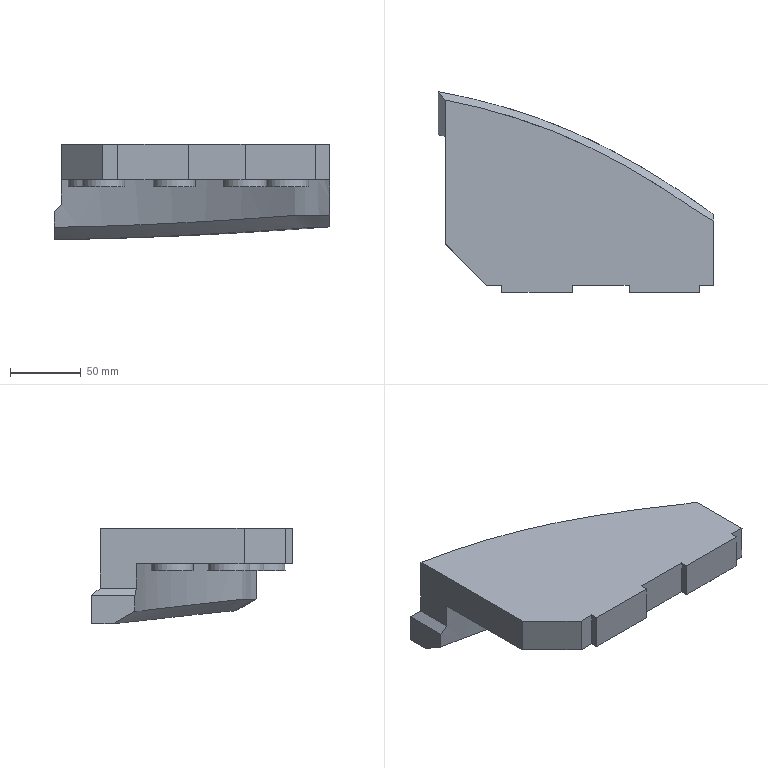Part | NX | features solid 2 | 1 solid | 32 faces | box 194.992 x 141.855 x 67.445 mm | volume 690689 mm3 | plane 21 | spline 6 | cylinder 5 | commonest cylinder face diameters 30 x5